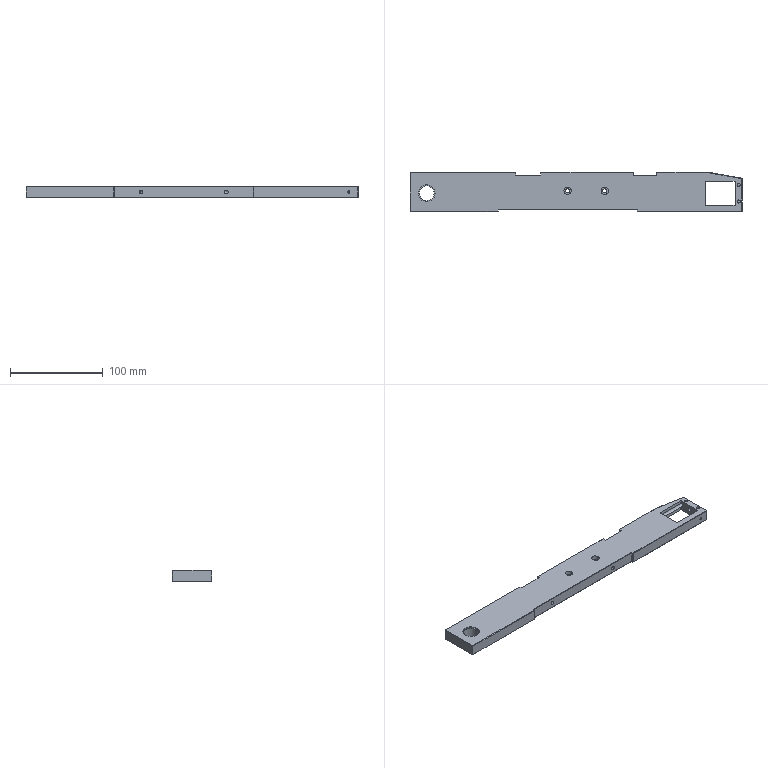Part | NX | features BREP 1 | 1 solid | 159 faces | box 358 x 42.5 x 12 mm | volume 159742 mm3 | plane 70 | cylinder 57 | cone 32 | commonest cylinder face diameters 3.3 x18 1 x8 5 x8 4.2 x6 4.3 x4 8 x4